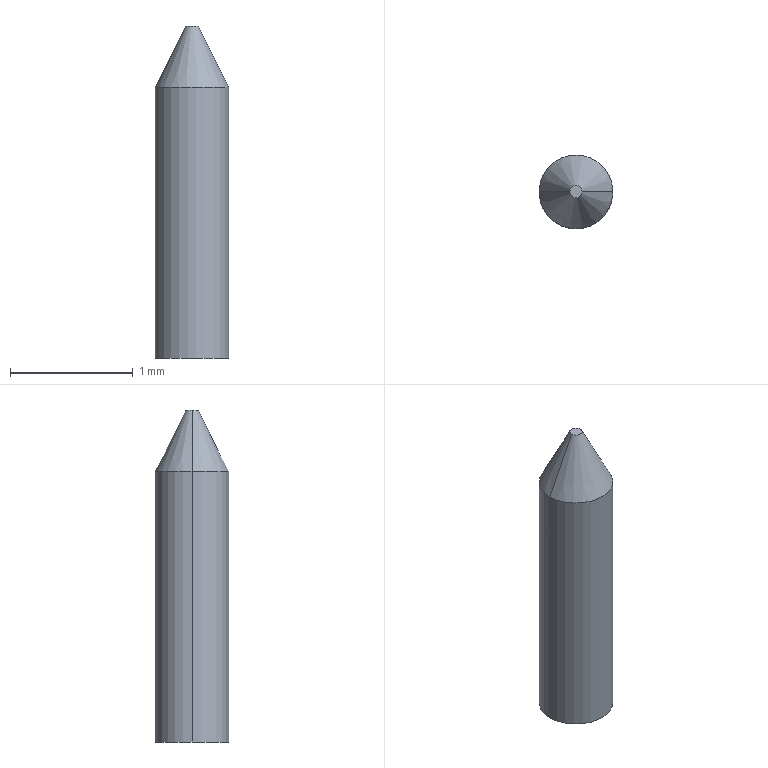Part | STEP file | 03-33 limit pin | 1 solid | 6 faces | box 0.6 x 0.6 x 2.7 mm | volume 0.6783 mm3 | cone 2 | cylinder 2 | plane 2 | commonest cylinder face diameters 0.6 x2
STEP:
#1=CARTESIAN_POINT('',(0.05,0.,2.7));
#2=VERTEX_POINT('',#1);
#3=CARTESIAN_POINT('',(-0.05,0.,2.7));
#4=VERTEX_POINT('',#3);
#5=CARTESIAN_POINT('',(0.,0.,2.7));
#6=DIRECTION('',(0.,0.,1.));
#7=DIRECTION('',(1.,0.,0.));
#8=AXIS2_PLACEMENT_3D('',#5,#6,#7);
#9=CIRCLE('',#8,0.05);
#10=EDGE_CURVE('',#2,#4,#9,.T.);
#11=ORIENTED_EDGE('',*,*,#10,.F.);
#12=CARTESIAN_POINT('',(0.3,0.,2.2));
#13=VERTEX_POINT('',#12);
#14=CARTESIAN_POINT('',(0.05,0.,2.7));
#15=DIRECTION('',(0.4472,0.,-0.8944));
#16=VECTOR('',#15,1000.);
#17=LINE('',#14,#16);
#18=EDGE_CURVE('',#2,#13,#17,.T.);
#19=ORIENTED_EDGE('',*,*,#18,.T.);
#20=CARTESIAN_POINT('',(-0.3,0.,2.2));
#21=VERTEX_POINT('',#20);
#22=CARTESIAN_POINT('',(0.,0.,2.2));
#23=DIRECTION('',(0.,0.,-1.));
#24=DIRECTION('',(1.,0.,0.));
#25=AXIS2_PLACEMENT_3D('',#22,#23,#24);
#26=CIRCLE('',#25,0.3);
#27=EDGE_CURVE('',#21,#13,#26,.T.);
#28=ORIENTED_EDGE('',*,*,#27,.F.);
#29=CARTESIAN_POINT('',(-0.05,0.,2.7));
#30=DIRECTION('',(-0.4472,0.,-0.8944));
#31=VECTOR('',#30,1000.);
#32=LINE('',#29,#31);
#33=EDGE_CURVE('',#4,#21,#32,.T.);
#34=ORIENTED_EDGE('',*,*,#33,.F.);
#35=EDGE_LOOP('',(#11,#19,#28,#34));
#36=FACE_OUTER_BOUND('',#35,.T.);
#37=CARTESIAN_POINT('',(0.,0.,2.7));
#38=DIRECTION('',(0.,0.,-1.));
#39=DIRECTION('',(-1.,0.,0.));
#40=AXIS2_PLACEMENT_3D('',#37,#38,#39);
#41=CONICAL_SURFACE('',#40,0.05,0.4636);
#42=ADVANCED_FACE('',(#36),#41,.T.);
#43=ORIENTED_EDGE('',*,*,#27,.T.);
#44=CARTESIAN_POINT('',(0.3,0.,0.));
#45=VERTEX_POINT('',#44);
#46=CARTESIAN_POINT('',(0.3,0.,2.7));
#47=DIRECTION('',(0.,0.,-1.));
#48=VECTOR('',#47,1000.);
#49=LINE('',#46,#48);
#50=EDGE_CURVE('',#13,#45,#49,.T.);
#51=ORIENTED_EDGE('',*,*,#50,.T.);
#52=CARTESIAN_POINT('',(-0.3,0.,0.));
#53=VERTEX_POINT('',#52);
#54=CARTESIAN_POINT('',(0.,0.,0.));
#55=DIRECTION('',(0.,0.,1.));
#56=DIRECTION('',(1.,0.,0.));
#57=AXIS2_PLACEMENT_3D('',#54,#55,#56);
#58=CIRCLE('',#57,0.3);
#59=EDGE_CURVE('',#45,#53,#58,.T.);
#60=ORIENTED_EDGE('',*,*,#59,.T.);
#61=CARTESIAN_POINT('',(-0.3,0.,2.7));
#62=DIRECTION('',(0.,0.,-1.));
#63=VECTOR('',#62,1000.);
#64=LINE('',#61,#63);
#65=EDGE_CURVE('',#21,#53,#64,.T.);
#66=ORIENTED_EDGE('',*,*,#65,.F.);
#67=EDGE_LOOP('',(#43,#51,#60,#66));
#68=FACE_OUTER_BOUND('',#67,.T.);
#69=CARTESIAN_POINT('',(0.,0.,2.7));
#70=DIRECTION('',(0.,0.,-1.));
#71=DIRECTION('',(-1.,0.,0.));
#72=AXIS2_PLACEMENT_3D('',#69,#70,#71);
#73=CYLINDRICAL_SURFACE('',#72,0.3);
#74=ADVANCED_FACE('',(#68),#73,.T.);
#75=ORIENTED_EDGE('',*,*,#50,.F.);
#76=CARTESIAN_POINT('',(0.,0.,2.2));
#77=DIRECTION('',(0.,0.,-1.));
#78=DIRECTION('',(1.,0.,0.));
#79=AXIS2_PLACEMENT_3D('',#76,#77,#78);
#80=CIRCLE('',#79,0.3);
#81=EDGE_CURVE('',#13,#21,#80,.T.);
#82=ORIENTED_EDGE('',*,*,#81,.T.);
#83=ORIENTED_EDGE('',*,*,#65,.T.);
#84=CARTESIAN_POINT('',(0.,0.,0.));
#85=DIRECTION('',(0.,0.,1.));
#86=DIRECTION('',(1.,0.,0.));
#87=AXIS2_PLACEMENT_3D('',#84,#85,#86);
#88=CIRCLE('',#87,0.3);
#89=EDGE_CURVE('',#53,#45,#88,.T.);
#90=ORIENTED_EDGE('',*,*,#89,.T.);
#91=EDGE_LOOP('',(#75,#82,#83,#90));
#92=FACE_OUTER_BOUND('',#91,.T.);
#93=CARTESIAN_POINT('',(0.,0.,2.7));
#94=DIRECTION('',(0.,0.,-1.));
#95=DIRECTION('',(-1.,0.,0.));
#96=AXIS2_PLACEMENT_3D('',#93,#94,#95);
#97=CYLINDRICAL_SURFACE('',#96,0.3);
#98=ADVANCED_FACE('',(#92),#97,.T.);
#99=CARTESIAN_POINT('',(0.,0.,2.7));
#100=DIRECTION('',(0.,0.,1.));
#101=DIRECTION('',(1.,0.,0.));
#102=AXIS2_PLACEMENT_3D('',#99,#100,#101);
#103=CIRCLE('',#102,0.05);
#104=EDGE_CURVE('',#4,#2,#103,.T.);
#105=ORIENTED_EDGE('',*,*,#104,.T.);
#106=ORIENTED_EDGE('',*,*,#10,.T.);
#107=EDGE_LOOP('',(#105,#106));
#108=FACE_OUTER_BOUND('',#107,.T.);
#109=CARTESIAN_POINT('',(0.,0.,2.7));
#110=DIRECTION('',(0.,0.,1.));
#111=DIRECTION('',(1.,0.,0.));
#112=AXIS2_PLACEMENT_3D('',#109,#110,#111);
#113=PLANE('',#112);
#114=ADVANCED_FACE('',(#108),#113,.T.);
#115=ORIENTED_EDGE('',*,*,#89,.F.);
#116=ORIENTED_EDGE('',*,*,#59,.F.);
#117=EDGE_LOOP('',(#115,#116));
#118=FACE_OUTER_BOUND('',#117,.T.);
#119=CARTESIAN_POINT('',(0.,0.,0.));
#120=DIRECTION('',(0.,0.,1.));
#121=DIRECTION('',(1.,0.,0.));
#122=AXIS2_PLACEMENT_3D('',#119,#120,#121);
#123=PLANE('',#122);
#124=ADVANCED_FACE('',(#118),#123,.F.);
#125=ORIENTED_EDGE('',*,*,#18,.F.);
#126=ORIENTED_EDGE('',*,*,#104,.F.);
#127=ORIENTED_EDGE('',*,*,#33,.T.);
#128=ORIENTED_EDGE('',*,*,#81,.F.);
#129=EDGE_LOOP('',(#125,#126,#127,#128));
#130=FACE_OUTER_BOUND('',#129,.T.);
#131=CARTESIAN_POINT('',(0.,0.,2.7));
#132=DIRECTION('',(0.,0.,-1.));
#133=DIRECTION('',(-1.,0.,0.));
#134=AXIS2_PLACEMENT_3D('',#131,#132,#133);
#135=CONICAL_SURFACE('',#134,0.05,0.4636);
#136=ADVANCED_FACE('',(#130),#135,.T.);
#137=CLOSED_SHELL('',(#42,#74,#98,#114,#124,#136));
#138=MANIFOLD_SOLID_BREP('',#137);
#139=CARTESIAN_POINT('',(0.,0.,0.));
#140=DIRECTION('',(0.,0.,1.));
#141=DIRECTION('',(1.,0.,0.));
#142=AXIS2_PLACEMENT_3D('',#139,#140,#141);
#143=(LENGTH_UNIT()NAMED_UNIT(*)SI_UNIT(.MILLI.,.METRE.));
#144=UNCERTAINTY_MEASURE_WITH_UNIT(LENGTH_MEASURE(0.00001),#143,'','');
#145=(NAMED_UNIT(*)PLANE_ANGLE_UNIT()SI_UNIT($,.RADIAN.));
#146=(NAMED_UNIT(*)SI_UNIT($,.STERADIAN.)SOLID_ANGLE_UNIT());
#147=(GEOMETRIC_REPRESENTATION_CONTEXT(3)GLOBAL_UNCERTAINTY_ASSIGNED_CONTEXT((#144))GLOBAL_UNIT_ASSIGNED_CONTEXT((#143,#145,#146))REPRESENTATION_CONTEXT('',''));
#148=ADVANCED_BREP_SHAPE_REPRESENTATION('',(#138,#142),#147);